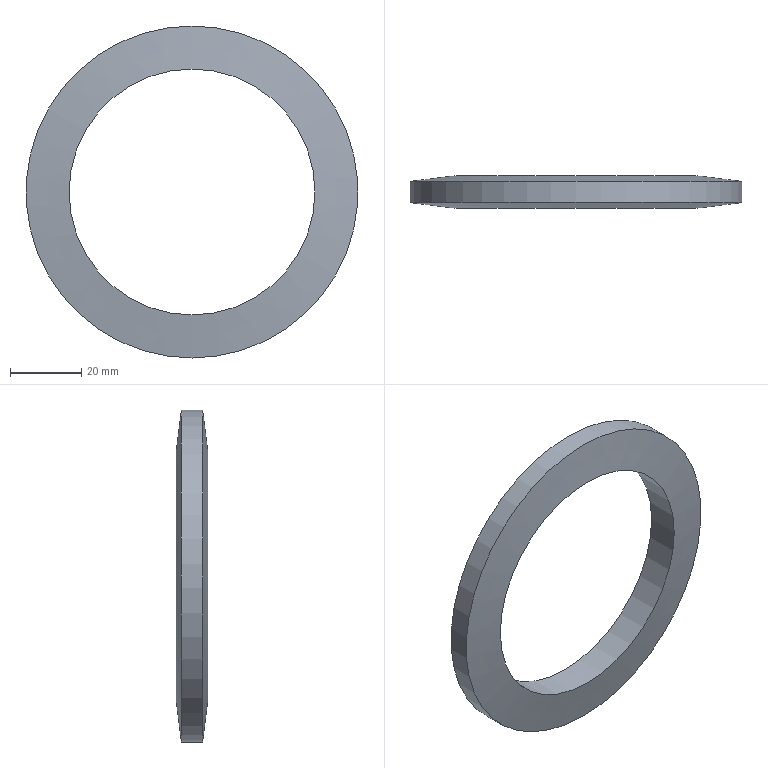Part | NX | features DATUM_CSYS 3, SKETCH 2, EXTRUDE 1, SWP104 1 | 1 solid | 4 faces | box 93.171 x 8.968 x 93.171 mm | volume 22814 mm3 | cone 2 | cylinder 2 | commonest cylinder face diameters 69 x1 93.171 x1
STEP:
#1=CARTESIAN_POINT('',(0.,-3.,-46.586));
#2=VERTEX_POINT('',#1);
#3=CARTESIAN_POINT('',(0.,-3.,0.));
#4=DIRECTION('',(0.,-1.,0.));
#5=DIRECTION('',(0.,0.,-1.));
#6=AXIS2_PLACEMENT_3D('',#3,#4,#5);
#7=CIRCLE('',#6,46.586);
#8=EDGE_CURVE('',#2,#2,#7,.T.);
#9=ORIENTED_EDGE('',*,*,#8,.T.);
#10=EDGE_LOOP('',(#9));
#11=FACE_BOUND('',#10,.T.);
#12=CARTESIAN_POINT('',(0.,-4.484,34.5));
#13=VERTEX_POINT('',#12);
#14=CARTESIAN_POINT('',(0.,-4.484,0.));
#15=DIRECTION('',(0.,1.,0.));
#16=DIRECTION('',(0.,0.,1.));
#17=AXIS2_PLACEMENT_3D('',#14,#15,#16);
#18=CIRCLE('',#17,34.5);
#19=EDGE_CURVE('',#13,#13,#18,.F.);
#20=ORIENTED_EDGE('',*,*,#19,.F.);
#21=EDGE_LOOP('',(#20));
#22=FACE_BOUND('',#21,.T.);
#23=CARTESIAN_POINT('',(0.,-3.,0.));
#24=DIRECTION('',(0.,1.,0.));
#25=DIRECTION('',(0.,0.,1.));
#26=AXIS2_PLACEMENT_3D('',#23,#24,#25);
#27=CONICAL_SURFACE('',#26,46.586,1.449);
#28=ADVANCED_FACE('',(#11,#22),#27,.T.);
#29=CARTESIAN_POINT('',(0.,3.,-46.586));
#30=VERTEX_POINT('',#29);
#31=CARTESIAN_POINT('',(0.,3.,0.));
#32=DIRECTION('',(0.,-1.,0.));
#33=DIRECTION('',(0.,0.,-1.));
#34=AXIS2_PLACEMENT_3D('',#31,#32,#33);
#35=CIRCLE('',#34,46.586);
#36=EDGE_CURVE('',#30,#30,#35,.T.);
#37=ORIENTED_EDGE('',*,*,#36,.F.);
#38=EDGE_LOOP('',(#37));
#39=FACE_BOUND('',#38,.T.);
#40=CARTESIAN_POINT('',(0.,4.484,-34.5));
#41=VERTEX_POINT('',#40);
#42=CARTESIAN_POINT('',(0.,4.484,0.));
#43=DIRECTION('',(0.,-1.,0.));
#44=DIRECTION('',(0.,0.,-1.));
#45=AXIS2_PLACEMENT_3D('',#42,#43,#44);
#46=CIRCLE('',#45,34.5);
#47=EDGE_CURVE('',#41,#41,#46,.F.);
#48=ORIENTED_EDGE('',*,*,#47,.F.);
#49=EDGE_LOOP('',(#48));
#50=FACE_BOUND('',#49,.T.);
#51=CARTESIAN_POINT('',(0.,8.72,0.));
#52=DIRECTION('',(0.,-1.,0.));
#53=DIRECTION('',(0.,0.,-1.));
#54=AXIS2_PLACEMENT_3D('',#51,#52,#53);
#55=CONICAL_SURFACE('',#54,0.,1.449);
#56=ADVANCED_FACE('',(#39,#50),#55,.T.);
#57=ORIENTED_EDGE('',*,*,#8,.F.);
#58=EDGE_LOOP('',(#57));
#59=FACE_BOUND('',#58,.T.);
#60=ORIENTED_EDGE('',*,*,#36,.T.);
#61=EDGE_LOOP('',(#60));
#62=FACE_BOUND('',#61,.T.);
#63=CARTESIAN_POINT('',(0.,0.,0.));
#64=DIRECTION('',(0.,-1.,0.));
#65=DIRECTION('',(0.,0.,-1.));
#66=AXIS2_PLACEMENT_3D('',#63,#64,#65);
#67=CYLINDRICAL_SURFACE('',#66,46.586);
#68=ADVANCED_FACE('',(#59,#62),#67,.T.);
#69=ORIENTED_EDGE('',*,*,#47,.T.);
#70=EDGE_LOOP('',(#69));
#71=FACE_BOUND('',#70,.T.);
#72=ORIENTED_EDGE('',*,*,#19,.T.);
#73=EDGE_LOOP('',(#72));
#74=FACE_BOUND('',#73,.T.);
#75=CARTESIAN_POINT('',(0.,125.,0.));
#76=DIRECTION('',(0.,-1.,0.));
#77=DIRECTION('',(0.,0.,-1.));
#78=AXIS2_PLACEMENT_3D('',#75,#76,#77);
#79=CYLINDRICAL_SURFACE('',#78,34.5);
#80=ADVANCED_FACE('',(#71,#74),#79,.F.);
#81=CLOSED_SHELL('',(#28,#56,#68,#80));
#82=MANIFOLD_SOLID_BREP('',#81);
#83=(LENGTH_UNIT()NAMED_UNIT(*)SI_UNIT(.MILLI.,.METRE.));
#84=UNCERTAINTY_MEASURE_WITH_UNIT(LENGTH_MEASURE(0.00001),#83,'','');
#85=(NAMED_UNIT(*)PLANE_ANGLE_UNIT()SI_UNIT($,.RADIAN.));
#86=(NAMED_UNIT(*)SI_UNIT($,.STERADIAN.)SOLID_ANGLE_UNIT());
#87=(GEOMETRIC_REPRESENTATION_CONTEXT(3)GLOBAL_UNCERTAINTY_ASSIGNED_CONTEXT((#84))GLOBAL_UNIT_ASSIGNED_CONTEXT((#83,#85,#86))REPRESENTATION_CONTEXT('',''));
#88=ADVANCED_BREP_SHAPE_REPRESENTATION('',(#82),#87);